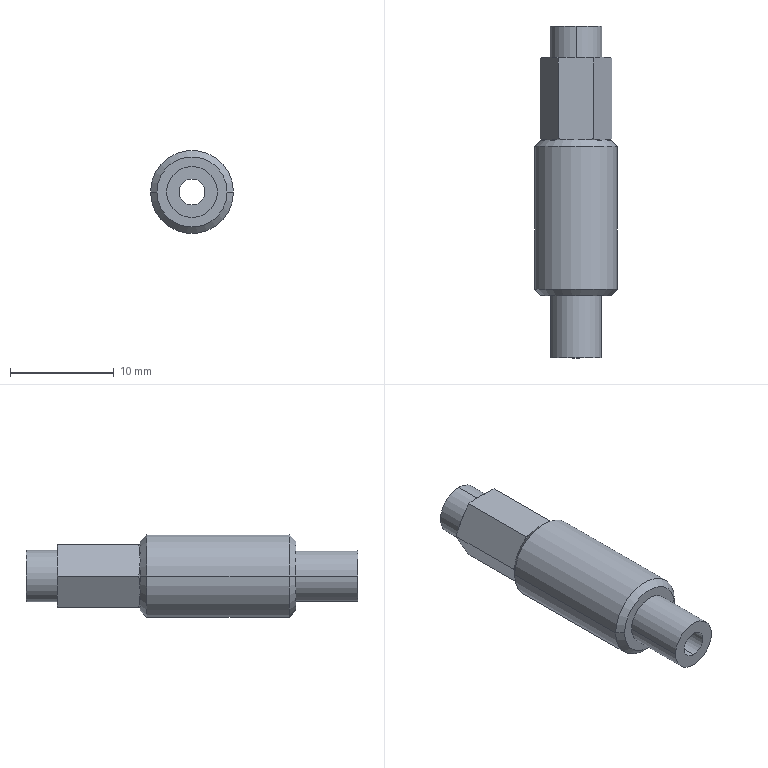Part | SolidWorks | features RefAxis 12, 3DProfileFeature 4, Revolution 2, ICE 1, RevCut 1 | 1 solid | 37 faces | box 8 x 32 x 8 mm | volume 1009 mm3 | cone 18 | plane 11 | cylinder 8 | commonest cylinder face diameters 2.5 x2 4.9 x2 5 x2 8 x2
STEP:
#1=CARTESIAN_POINT('',(0.,12.,-1.25));
#2=VERTEX_POINT('',#1);
#3=CARTESIAN_POINT('',(0.,12.,1.25));
#4=VERTEX_POINT('',#3);
#5=CARTESIAN_POINT('',(0.,12.,0.));
#6=DIRECTION('',(0.,1.,0.));
#7=DIRECTION('',(0.,0.,1.));
#8=AXIS2_PLACEMENT_3D('',#5,#6,#7);
#9=CIRCLE('',#8,1.25);
#10=EDGE_CURVE('',#2,#4,#9,.T.);
#11=ORIENTED_EDGE('',*,*,#10,.F.);
#12=CARTESIAN_POINT('',(0.,44.,-1.25));
#13=VERTEX_POINT('',#12);
#14=CARTESIAN_POINT('',(0.,12.,-1.25));
#15=DIRECTION('',(0.,1.,0.));
#16=VECTOR('',#15,1000.);
#17=LINE('',#14,#16);
#18=EDGE_CURVE('',#2,#13,#17,.T.);
#19=ORIENTED_EDGE('',*,*,#18,.T.);
#20=CARTESIAN_POINT('',(0.,44.,1.25));
#21=VERTEX_POINT('',#20);
#22=CARTESIAN_POINT('',(0.,44.,0.));
#23=DIRECTION('',(0.,1.,0.));
#24=DIRECTION('',(0.,0.,1.));
#25=AXIS2_PLACEMENT_3D('',#22,#23,#24);
#26=CIRCLE('',#25,1.25);
#27=EDGE_CURVE('',#13,#21,#26,.T.);
#28=ORIENTED_EDGE('',*,*,#27,.T.);
#29=CARTESIAN_POINT('',(0.,12.,1.25));
#30=DIRECTION('',(0.,1.,0.));
#31=VECTOR('',#30,1000.);
#32=LINE('',#29,#31);
#33=EDGE_CURVE('',#4,#21,#32,.T.);
#34=ORIENTED_EDGE('',*,*,#33,.F.);
#35=EDGE_LOOP('',(#11,#19,#28,#34));
#36=FACE_OUTER_BOUND('',#35,.T.);
#37=CARTESIAN_POINT('',(0.,12.,0.));
#38=DIRECTION('',(0.,1.,0.));
#39=DIRECTION('',(0.,0.,1.));
#40=AXIS2_PLACEMENT_3D('',#37,#38,#39);
#41=CYLINDRICAL_SURFACE('',#40,1.25);
#42=ADVANCED_FACE('',(#36),#41,.F.);
#43=CARTESIAN_POINT('',(0.,41.,2.5));
#44=VERTEX_POINT('',#43);
#45=CARTESIAN_POINT('',(0.,41.,-2.5));
#46=VERTEX_POINT('',#45);
#47=CARTESIAN_POINT('',(0.,41.,0.));
#48=DIRECTION('',(0.,1.,0.));
#49=DIRECTION('',(1.,0.,0.));
#50=AXIS2_PLACEMENT_3D('',#47,#48,#49);
#51=CIRCLE('',#50,2.5);
#52=EDGE_CURVE('',#44,#46,#51,.T.);
#53=ORIENTED_EDGE('',*,*,#52,.T.);
#54=CARTESIAN_POINT('',(0.,44.,-2.5));
#55=VERTEX_POINT('',#54);
#56=CARTESIAN_POINT('',(0.,41.,-2.5));
#57=DIRECTION('',(0.,1.,0.));
#58=VECTOR('',#57,1000.);
#59=LINE('',#56,#58);
#60=EDGE_CURVE('',#46,#55,#59,.T.);
#61=ORIENTED_EDGE('',*,*,#60,.T.);
#62=CARTESIAN_POINT('',(0.,44.,2.5));
#63=VERTEX_POINT('',#62);
#64=CARTESIAN_POINT('',(0.,44.,0.));
#65=DIRECTION('',(0.,1.,0.));
#66=DIRECTION('',(0.,0.,1.));
#67=AXIS2_PLACEMENT_3D('',#64,#65,#66);
#68=CIRCLE('',#67,2.5);
#69=EDGE_CURVE('',#63,#55,#68,.T.);
#70=ORIENTED_EDGE('',*,*,#69,.F.);
#71=CARTESIAN_POINT('',(0.,41.,2.5));
#72=DIRECTION('',(0.,1.,0.));
#73=VECTOR('',#72,1000.);
#74=LINE('',#71,#73);
#75=EDGE_CURVE('',#44,#63,#74,.T.);
#76=ORIENTED_EDGE('',*,*,#75,.F.);
#77=EDGE_LOOP('',(#53,#61,#70,#76));
#78=FACE_OUTER_BOUND('',#77,.T.);
#79=CARTESIAN_POINT('',(0.,41.,0.));
#80=DIRECTION('',(0.,1.,0.));
#81=DIRECTION('',(0.,0.,1.));
#82=AXIS2_PLACEMENT_3D('',#79,#80,#81);
#83=CYLINDRICAL_SURFACE('',#82,2.5);
#84=ADVANCED_FACE('',(#78),#83,.T.);
#85=CARTESIAN_POINT('',(3.,41.,0.));
#86=VERTEX_POINT('',#85);
#87=CARTESIAN_POINT('',(2.598,41.,-1.5));
#88=VERTEX_POINT('',#87);
#89=CARTESIAN_POINT('',(0.,41.,0.));
#90=DIRECTION('',(0.,1.,0.));
#91=DIRECTION('',(-1.,0.,0.));
#92=AXIS2_PLACEMENT_3D('',#89,#90,#91);
#93=CIRCLE('',#92,3.);
#94=EDGE_CURVE('',#86,#88,#93,.T.);
#95=ORIENTED_EDGE('',*,*,#94,.F.);
#96=CARTESIAN_POINT('',(3.464,40.918,0.));
#97=VERTEX_POINT('',#96);
#98=CARTESIAN_POINT('',(5.,40.647,0.));
#99=DIRECTION('',(0.9848,-0.1736,0.));
#100=VECTOR('',#99,1000.);
#101=LINE('',#98,#100);
#102=EDGE_CURVE('',#86,#97,#101,.T.);
#103=ORIENTED_EDGE('',*,*,#102,.T.);
#104=CARTESIAN_POINT('',(3.464,40.918,0.));
#105=CARTESIAN_POINT('',(3.175,40.969,-0.5));
#106=CARTESIAN_POINT('',(2.887,41.,-1.));
#107=CARTESIAN_POINT('',(2.598,41.,-1.5));
#108=B_SPLINE_CURVE_WITH_KNOTS('',3,(#104,#105,#106,#107),.UNSPECIFIED.,.F.,.F.,(4,4),(0.000000231,0.001732),.UNSPECIFIED.);
#109=EDGE_CURVE('',#97,#88,#108,.T.);
#110=ORIENTED_EDGE('',*,*,#109,.T.);
#111=EDGE_LOOP('',(#95,#103,#110));
#112=FACE_OUTER_BOUND('',#111,.T.);
#113=CARTESIAN_POINT('',(0.,40.647,0.));
#114=DIRECTION('',(0.,-1.,0.));
#115=DIRECTION('',(1.,0.,0.));
#116=AXIS2_PLACEMENT_3D('',#113,#114,#115);
#117=CONICAL_SURFACE('',#116,5.,1.396);
#118=ADVANCED_FACE('',(#112),#117,.T.);
#119=CARTESIAN_POINT('',(-2.45,12.,0.));
#120=VERTEX_POINT('',#119);
#121=CARTESIAN_POINT('',(2.45,12.,0.));
#122=VERTEX_POINT('',#121);
#123=CARTESIAN_POINT('',(0.,12.,0.));
#124=DIRECTION('',(0.,1.,0.));
#125=DIRECTION('',(-1.,0.,0.));
#126=AXIS2_PLACEMENT_3D('',#123,#124,#125);
#127=CIRCLE('',#126,2.45);
#128=EDGE_CURVE('',#120,#122,#127,.T.);
#129=ORIENTED_EDGE('',*,*,#128,.T.);
#130=CARTESIAN_POINT('',(2.45,18.,0.));
#131=VERTEX_POINT('',#130);
#132=CARTESIAN_POINT('',(2.45,12.,0.));
#133=DIRECTION('',(0.,1.,0.));
#134=VECTOR('',#133,1000.);
#135=LINE('',#132,#134);
#136=EDGE_CURVE('',#122,#131,#135,.T.);
#137=ORIENTED_EDGE('',*,*,#136,.T.);
#138=CARTESIAN_POINT('',(-2.45,18.,0.));
#139=VERTEX_POINT('',#138);
#140=CARTESIAN_POINT('',(0.,18.,0.));
#141=DIRECTION('',(0.,1.,0.));
#142=DIRECTION('',(-1.,0.,0.));
#143=AXIS2_PLACEMENT_3D('',#140,#141,#142);
#144=CIRCLE('',#143,2.45);
#145=EDGE_CURVE('',#139,#131,#144,.T.);
#146=ORIENTED_EDGE('',*,*,#145,.F.);
#147=CARTESIAN_POINT('',(-2.45,12.,0.));
#148=DIRECTION('',(0.,1.,0.));
#149=VECTOR('',#148,1000.);
#150=LINE('',#147,#149);
#151=EDGE_CURVE('',#120,#139,#150,.T.);
#152=ORIENTED_EDGE('',*,*,#151,.F.);
#153=EDGE_LOOP('',(#129,#137,#146,#152));
#154=FACE_OUTER_BOUND('',#153,.T.);
#155=CARTESIAN_POINT('',(0.,12.,0.));
#156=DIRECTION('',(0.,1.,0.));
#157=DIRECTION('',(-1.,0.,0.));
#158=AXIS2_PLACEMENT_3D('',#155,#156,#157);
#159=CYLINDRICAL_SURFACE('',#158,2.45);
#160=ADVANCED_FACE('',(#154),#159,.T.);
#161=CARTESIAN_POINT('',(-3.387,18.,0.));
#162=VERTEX_POINT('',#161);
#163=CARTESIAN_POINT('',(3.386,18.,0.));
#164=VERTEX_POINT('',#163);
#165=CARTESIAN_POINT('',(0.,18.,0.));
#166=DIRECTION('',(0.,1.,0.));
#167=DIRECTION('',(-1.,0.,0.));
#168=AXIS2_PLACEMENT_3D('',#165,#166,#167);
#169=CIRCLE('',#168,3.387);
#170=EDGE_CURVE('',#162,#164,#169,.T.);
#171=ORIENTED_EDGE('',*,*,#170,.T.);
#172=CARTESIAN_POINT('',(4.,18.614,0.));
#173=VERTEX_POINT('',#172);
#174=CARTESIAN_POINT('',(3.386,18.,0.));
#175=DIRECTION('',(0.7071,0.7071,0.));
#176=VECTOR('',#175,1000.);
#177=LINE('',#174,#176);
#178=EDGE_CURVE('',#164,#173,#177,.T.);
#179=ORIENTED_EDGE('',*,*,#178,.T.);
#180=CARTESIAN_POINT('',(-4.,18.614,0.));
#181=VERTEX_POINT('',#180);
#182=CARTESIAN_POINT('',(0.,18.614,0.));
#183=DIRECTION('',(0.,1.,0.));
#184=DIRECTION('',(-1.,0.,0.));
#185=AXIS2_PLACEMENT_3D('',#182,#183,#184);
#186=CIRCLE('',#185,4.);
#187=EDGE_CURVE('',#181,#173,#186,.T.);
#188=ORIENTED_EDGE('',*,*,#187,.F.);
#189=CARTESIAN_POINT('',(-3.387,18.,0.));
#190=DIRECTION('',(-0.7071,0.7071,0.));
#191=VECTOR('',#190,1000.);
#192=LINE('',#189,#191);
#193=EDGE_CURVE('',#162,#181,#192,.T.);
#194=ORIENTED_EDGE('',*,*,#193,.F.);
#195=EDGE_LOOP('',(#171,#179,#188,#194));
#196=FACE_OUTER_BOUND('',#195,.T.);
#197=CARTESIAN_POINT('',(0.,18.,0.));
#198=DIRECTION('',(0.,1.,0.));
#199=DIRECTION('',(-1.,0.,0.));
#200=AXIS2_PLACEMENT_3D('',#197,#198,#199);
#201=CONICAL_SURFACE('',#200,3.387,0.7854);
#202=ADVANCED_FACE('',(#196),#201,.T.);
#203=ORIENTED_EDGE('',*,*,#187,.T.);
#204=CARTESIAN_POINT('',(4.,32.386,0.));
#205=VERTEX_POINT('',#204);
#206=CARTESIAN_POINT('',(4.,12.,0.));
#207=DIRECTION('',(0.,1.,0.));
#208=VECTOR('',#207,1000.);
#209=LINE('',#206,#208);
#210=EDGE_CURVE('',#173,#205,#209,.T.);
#211=ORIENTED_EDGE('',*,*,#210,.T.);
#212=CARTESIAN_POINT('',(-4.,32.386,0.));
#213=VERTEX_POINT('',#212);
#214=CARTESIAN_POINT('',(0.,32.386,0.));
#215=DIRECTION('',(0.,1.,0.));
#216=DIRECTION('',(-1.,0.,0.));
#217=AXIS2_PLACEMENT_3D('',#214,#215,#216);
#218=CIRCLE('',#217,4.);
#219=EDGE_CURVE('',#213,#205,#218,.T.);
#220=ORIENTED_EDGE('',*,*,#219,.F.);
#221=CARTESIAN_POINT('',(-4.,12.,0.));
#222=DIRECTION('',(0.,1.,0.));
#223=VECTOR('',#222,1000.);
#224=LINE('',#221,#223);
#225=EDGE_CURVE('',#181,#213,#224,.T.);
#226=ORIENTED_EDGE('',*,*,#225,.F.);
#227=EDGE_LOOP('',(#203,#211,#220,#226));
#228=FACE_OUTER_BOUND('',#227,.T.);
#229=CARTESIAN_POINT('',(0.,12.,0.));
#230=DIRECTION('',(0.,1.,0.));
#231=DIRECTION('',(-1.,0.,0.));
#232=AXIS2_PLACEMENT_3D('',#229,#230,#231);
#233=CYLINDRICAL_SURFACE('',#232,4.);
#234=ADVANCED_FACE('',(#228),#233,.T.);
#235=CARTESIAN_POINT('',(-3.387,33.,0.));
#236=VERTEX_POINT('',#235);
#237=CARTESIAN_POINT('',(3.387,33.,0.));
#238=VERTEX_POINT('',#237);
#239=CARTESIAN_POINT('',(0.,33.,0.));
#240=DIRECTION('',(0.,1.,0.));
#241=DIRECTION('',(-1.,0.,0.));
#242=AXIS2_PLACEMENT_3D('',#239,#240,#241);
#243=CIRCLE('',#242,3.387);
#244=EDGE_CURVE('',#236,#238,#243,.T.);
#245=ORIENTED_EDGE('',*,*,#244,.F.);
#246=CARTESIAN_POINT('',(-4.,32.386,0.));
#247=DIRECTION('',(-0.7071,-0.7071,0.));
#248=VECTOR('',#247,1000.);
#249=LINE('',#246,#248);
#250=EDGE_CURVE('',#236,#213,#249,.T.);
#251=ORIENTED_EDGE('',*,*,#250,.T.);
#252=ORIENTED_EDGE('',*,*,#219,.T.);
#253=CARTESIAN_POINT('',(4.,32.386,0.));
#254=DIRECTION('',(0.7071,-0.7071,0.));
#255=VECTOR('',#254,1000.);
#256=LINE('',#253,#255);
#257=EDGE_CURVE('',#238,#205,#256,.T.);
#258=ORIENTED_EDGE('',*,*,#257,.F.);
#259=EDGE_LOOP('',(#245,#251,#252,#258));
#260=FACE_OUTER_BOUND('',#259,.T.);
#261=CARTESIAN_POINT('',(0.,32.386,0.));
#262=DIRECTION('',(0.,-1.,0.));
#263=DIRECTION('',(1.,0.,0.));
#264=AXIS2_PLACEMENT_3D('',#261,#262,#263);
#265=CONICAL_SURFACE('',#264,4.,0.7854);
#266=ADVANCED_FACE('',(#260),#265,.T.);
#267=CARTESIAN_POINT('',(-2.598,33.,-1.5));
#268=VERTEX_POINT('',#267);
#269=CARTESIAN_POINT('',(-3.,33.,0.));
#270=VERTEX_POINT('',#269);
#271=CARTESIAN_POINT('',(0.,33.,0.));
#272=DIRECTION('',(0.,1.,0.));
#273=DIRECTION('',(-1.,0.,0.));
#274=AXIS2_PLACEMENT_3D('',#271,#272,#273);
#275=CIRCLE('',#274,3.);
#276=EDGE_CURVE('',#268,#270,#275,.T.);
#277=ORIENTED_EDGE('',*,*,#276,.T.);
#278=CARTESIAN_POINT('',(-3.464,33.124,0.));
#279=VERTEX_POINT('',#278);
#280=CARTESIAN_POINT('',(-3.,33.,0.));
#281=DIRECTION('',(-0.9659,0.2588,0.));
#282=VECTOR('',#281,1000.);
#283=LINE('',#280,#282);
#284=EDGE_CURVE('',#270,#279,#283,.T.);
#285=ORIENTED_EDGE('',*,*,#284,.T.);
#286=CARTESIAN_POINT('',(-3.464,33.124,0.));
#287=CARTESIAN_POINT('',(-3.175,33.047,-0.5));
#288=CARTESIAN_POINT('',(-2.887,33.,-1.));
#289=CARTESIAN_POINT('',(-2.598,33.,-1.5));
#290=B_SPLINE_CURVE_WITH_KNOTS('',3,(#286,#287,#288,#289),.UNSPECIFIED.,.F.,.F.,(4,4),(0.000000231,0.001732),.UNSPECIFIED.);
#291=EDGE_CURVE('',#279,#268,#290,.T.);
#292=ORIENTED_EDGE('',*,*,#291,.T.);
#293=EDGE_LOOP('',(#277,#285,#292));
#294=FACE_OUTER_BOUND('',#293,.T.);
#295=CARTESIAN_POINT('',(0.,33.,0.));
#296=DIRECTION('',(0.,1.,0.));
#297=DIRECTION('',(-1.,0.,0.));
#298=AXIS2_PLACEMENT_3D('',#295,#296,#297);
#299=CONICAL_SURFACE('',#298,3.,1.309);
#300=ADVANCED_FACE('',(#294),#299,.T.);
#301=ORIENTED_EDGE('',*,*,#128,.F.);
#302=CARTESIAN_POINT('',(0.,12.,0.));
#303=DIRECTION('',(0.,1.,0.));
#304=DIRECTION('',(-1.,0.,0.));
#305=AXIS2_PLACEMENT_3D('',#302,#303,#304);
#306=CIRCLE('',#305,2.45);
#307=EDGE_CURVE('',#122,#120,#306,.T.);
#308=ORIENTED_EDGE('',*,*,#307,.F.);
#309=EDGE_LOOP('',(#301,#308));
#310=FACE_OUTER_BOUND('',#309,.T.);
#311=CARTESIAN_POINT('',(0.,12.,0.));
#312=DIRECTION('',(0.,1.,0.));
#313=DIRECTION('',(0.,0.,1.));
#314=AXIS2_PLACEMENT_3D('',#311,#312,#313);
#315=CIRCLE('',#314,1.25);
#316=EDGE_CURVE('',#4,#2,#315,.T.);
#317=ORIENTED_EDGE('',*,*,#316,.T.);
#318=ORIENTED_EDGE('',*,*,#10,.T.);
#319=EDGE_LOOP('',(#317,#318));
#320=FACE_BOUND('',#319,.T.);
#321=CARTESIAN_POINT('',(2.45,12.,0.));
#322=DIRECTION('',(0.,1.,0.));
#323=DIRECTION('',(-1.,0.,0.));
#324=AXIS2_PLACEMENT_3D('',#321,#322,#323);
#325=PLANE('',#324);
#326=ADVANCED_FACE('',(#310,#320),#325,.F.);
#327=ORIENTED_EDGE('',*,*,#69,.T.);
#328=CARTESIAN_POINT('',(0.,44.,0.));
#329=DIRECTION('',(0.,1.,0.));
#330=DIRECTION('',(0.,0.,1.));
#331=AXIS2_PLACEMENT_3D('',#328,#329,#330);
#332=CIRCLE('',#331,2.5);
#333=EDGE_CURVE('',#55,#63,#332,.T.);
#334=ORIENTED_EDGE('',*,*,#333,.T.);
#335=EDGE_LOOP('',(#327,#334));
#336=FACE_OUTER_BOUND('',#335,.T.);
#337=CARTESIAN_POINT('',(0.,44.,0.));
#338=DIRECTION('',(0.,1.,0.));
#339=DIRECTION('',(0.,0.,1.));
#340=AXIS2_PLACEMENT_3D('',#337,#338,#339);
#341=CIRCLE('',#340,1.25);
#342=EDGE_CURVE('',#21,#13,#341,.T.);
#343=ORIENTED_EDGE('',*,*,#342,.F.);
#344=ORIENTED_EDGE('',*,*,#27,.F.);
#345=EDGE_LOOP('',(#343,#344));
#346=FACE_BOUND('',#345,.T.);
#347=CARTESIAN_POINT('',(0.,44.,0.));
#348=DIRECTION('',(0.,-1.,0.));
#349=DIRECTION('',(0.,0.,-1.));
#350=AXIS2_PLACEMENT_3D('',#347,#348,#349);
#351=PLANE('',#350);
#352=ADVANCED_FACE('',(#336,#346),#351,.F.);
#353=CARTESIAN_POINT('',(-2.598,41.,1.5));
#354=VERTEX_POINT('',#353);
#355=CARTESIAN_POINT('',(0.,41.,3.));
#356=VERTEX_POINT('',#355);
#357=CARTESIAN_POINT('',(0.,41.,0.));
#358=DIRECTION('',(0.,1.,0.));
#359=DIRECTION('',(-1.,0.,0.));
#360=AXIS2_PLACEMENT_3D('',#357,#358,#359);
#361=CIRCLE('',#360,3.);
#362=EDGE_CURVE('',#354,#356,#361,.T.);
#363=ORIENTED_EDGE('',*,*,#362,.T.);
#364=CARTESIAN_POINT('',(2.598,41.,1.5));
#365=VERTEX_POINT('',#364);
#366=CARTESIAN_POINT('',(0.,41.,0.));
#367=DIRECTION('',(0.,1.,0.));
#368=DIRECTION('',(-1.,0.,0.));
#369=AXIS2_PLACEMENT_3D('',#366,#367,#368);
#370=CIRCLE('',#369,3.);
#371=EDGE_CURVE('',#356,#365,#370,.T.);
#372=ORIENTED_EDGE('',*,*,#371,.T.);
#373=CARTESIAN_POINT('',(0.,41.,0.));
#374=DIRECTION('',(0.,1.,0.));
#375=DIRECTION('',(-1.,0.,0.));
#376=AXIS2_PLACEMENT_3D('',#373,#374,#375);
#377=CIRCLE('',#376,3.);
#378=EDGE_CURVE('',#365,#86,#377,.T.);
#379=ORIENTED_EDGE('',*,*,#378,.T.);
#380=ORIENTED_EDGE('',*,*,#94,.T.);
#381=CARTESIAN_POINT('',(0.,41.,-3.));
#382=VERTEX_POINT('',#381);
#383=CARTESIAN_POINT('',(0.,41.,0.));
#384=DIRECTION('',(0.,1.,0.));
#385=DIRECTION('',(-1.,0.,0.));
#386=AXIS2_PLACEMENT_3D('',#383,#384,#385);
#387=CIRCLE('',#386,3.);
#388=EDGE_CURVE('',#88,#382,#387,.T.);
#389=ORIENTED_EDGE('',*,*,#388,.T.);
#390=CARTESIAN_POINT('',(-2.598,41.,-1.5));
#391=VERTEX_POINT('',#390);
#392=CARTESIAN_POINT('',(0.,41.,0.));
#393=DIRECTION('',(0.,1.,0.));
#394=DIRECTION('',(-1.,0.,0.));
#395=AXIS2_PLACEMENT_3D('',#392,#393,#394);
#396=CIRCLE('',#395,3.);
#397=EDGE_CURVE('',#382,#391,#396,.T.);
#398=ORIENTED_EDGE('',*,*,#397,.T.);
#399=CARTESIAN_POINT('',(0.,41.,0.));
#400=DIRECTION('',(0.,1.,0.));
#401=DIRECTION('',(-1.,0.,0.));
#402=AXIS2_PLACEMENT_3D('',#399,#400,#401);
#403=CIRCLE('',#402,3.);
#404=EDGE_CURVE('',#391,#354,#403,.T.);
#405=ORIENTED_EDGE('',*,*,#404,.T.);
#406=EDGE_LOOP('',(#363,#372,#379,#380,#389,#398,#405));
#407=FACE_OUTER_BOUND('',#406,.T.);
#408=ORIENTED_EDGE('',*,*,#52,.F.);
#409=CARTESIAN_POINT('',(0.,41.,0.));
#410=DIRECTION('',(0.,1.,0.));
#411=DIRECTION('',(1.,0.,0.));
#412=AXIS2_PLACEMENT_3D('',#409,#410,#411);
#413=CIRCLE('',#412,2.5);
#414=EDGE_CURVE('',#46,#44,#413,.T.);
#415=ORIENTED_EDGE('',*,*,#414,.F.);
#416=EDGE_LOOP('',(#408,#415));
#417=FACE_BOUND('',#416,.T.);
#418=CARTESIAN_POINT('',(0.,41.,0.));
#419=DIRECTION('',(0.,-1.,0.));
#420=DIRECTION('',(1.,0.,0.));
#421=AXIS2_PLACEMENT_3D('',#418,#419,#420);
#422=PLANE('',#421);
#423=ADVANCED_FACE('',(#407,#417),#422,.F.);
#424=CARTESIAN_POINT('',(2.598,33.,1.5));
#425=VERTEX_POINT('',#424);
#426=CARTESIAN_POINT('',(1.732,33.124,3.));
#427=VERTEX_POINT('',#426);
#428=CARTESIAN_POINT('',(2.598,33.,1.5));
#429=CARTESIAN_POINT('',(2.309,33.,2.));
#430=CARTESIAN_POINT('',(2.021,33.047,2.5));
#431=CARTESIAN_POINT('',(1.732,33.124,3.));
#432=B_SPLINE_CURVE_WITH_KNOTS('',3,(#428,#429,#430,#431),.UNSPECIFIED.,.F.,.F.,(4,4),(0.001732,0.003464),.UNSPECIFIED.);
#433=EDGE_CURVE('',#425,#427,#432,.T.);
#434=ORIENTED_EDGE('',*,*,#433,.T.);
#435=CARTESIAN_POINT('',(0.,33.,3.));
#436=VERTEX_POINT('',#435);
#437=CARTESIAN_POINT('',(1.732,33.124,3.));
#438=CARTESIAN_POINT('',(1.156,33.047,3.));
#439=CARTESIAN_POINT('',(0.5785,33.,3.));
#440=CARTESIAN_POINT('',(0.,33.,3.));
#441=B_SPLINE_CURVE_WITH_KNOTS('',3,(#437,#438,#439,#440),.UNSPECIFIED.,.F.,.F.,(4,4),(0.00677,0.008513),.UNSPECIFIED.);
#442=EDGE_CURVE('',#427,#436,#441,.T.);
#443=ORIENTED_EDGE('',*,*,#442,.T.);
#444=CARTESIAN_POINT('',(0.,33.,0.));
#445=DIRECTION('',(0.,1.,0.));
#446=DIRECTION('',(-1.,0.,0.));
#447=AXIS2_PLACEMENT_3D('',#444,#445,#446);
#448=CIRCLE('',#447,3.);
#449=EDGE_CURVE('',#436,#425,#448,.T.);
#450=ORIENTED_EDGE('',*,*,#449,.T.);
#451=EDGE_LOOP('',(#434,#443,#450));
#452=FACE_OUTER_BOUND('',#451,.T.);
#453=CARTESIAN_POINT('',(0.,33.,0.));
#454=DIRECTION('',(0.,1.,0.));
#455=DIRECTION('',(-1.,0.,0.));
#456=AXIS2_PLACEMENT_3D('',#453,#454,#455);
#457=CONICAL_SURFACE('',#456,3.,1.309);
#458=ADVANCED_FACE('',(#452),#457,.T.);
#459=CARTESIAN_POINT('',(-2.598,33.,1.5));
#460=VERTEX_POINT('',#459);
#461=CARTESIAN_POINT('',(0.,33.,0.));
#462=DIRECTION('',(0.,1.,0.));
#463=DIRECTION('',(-1.,0.,0.));
#464=AXIS2_PLACEMENT_3D('',#461,#462,#463);
#465=CIRCLE('',#464,3.);
#466=EDGE_CURVE('',#460,#436,#465,.T.);
#467=ORIENTED_EDGE('',*,*,#466,.T.);
#468=CARTESIAN_POINT('',(-1.732,33.124,3.));
#469=VERTEX_POINT('',#468);
#470=CARTESIAN_POINT('',(0.,33.,3.));
#471=CARTESIAN_POINT('',(-0.5766,33.,3.));
#472=CARTESIAN_POINT('',(-1.156,33.047,3.));
#473=CARTESIAN_POINT('',(-1.732,33.124,3.));
#474=B_SPLINE_CURVE_WITH_KNOTS('',3,(#470,#471,#472,#473),.UNSPECIFIED.,.F.,.F.,(4,4),(0.008513,0.01025),.UNSPECIFIED.);
#475=EDGE_CURVE('',#436,#469,#474,.T.);
#476=ORIENTED_EDGE('',*,*,#475,.T.);
#477=CARTESIAN_POINT('',(-1.732,33.124,3.));
#478=CARTESIAN_POINT('',(-2.021,33.047,2.5));
#479=CARTESIAN_POINT('',(-2.309,33.,2.));
#480=CARTESIAN_POINT('',(-2.598,33.,1.5));
#481=B_SPLINE_CURVE_WITH_KNOTS('',3,(#477,#478,#479,#480),.UNSPECIFIED.,.F.,.F.,(4,4),(0.000000231,0.001732),.UNSPECIFIED.);
#482=EDGE_CURVE('',#469,#460,#481,.T.);
#483=ORIENTED_EDGE('',*,*,#482,.T.);
#484=EDGE_LOOP('',(#467,#476,#483));
#485=FACE_OUTER_BOUND('',#484,.T.);
#486=CARTESIAN_POINT('',(0.,33.,0.));
#487=DIRECTION('',(0.,1.,0.));
#488=DIRECTION('',(-1.,0.,0.));
#489=AXIS2_PLACEMENT_3D('',#486,#487,#488);
#490=CONICAL_SURFACE('',#489,3.,1.309);
#491=ADVANCED_FACE('',(#485),#490,.T.);
#492=ORIENTED_EDGE('',*,*,#284,.F.);
#493=CARTESIAN_POINT('',(0.,33.,0.));
#494=DIRECTION('',(0.,1.,0.));
#495=DIRECTION('',(-1.,0.,0.));
#496=AXIS2_PLACEMENT_3D('',#493,#494,#495);
#497=CIRCLE('',#496,3.);
#498=EDGE_CURVE('',#270,#460,#497,.T.);
#499=ORIENTED_EDGE('',*,*,#498,.T.);
#500=CARTESIAN_POINT('',(-2.598,33.,1.5));
#501=CARTESIAN_POINT('',(-2.887,33.,1.));
#502=CARTESIAN_POINT('',(-3.175,33.047,0.5));
#503=CARTESIAN_POINT('',(-3.464,33.124,0.));
#504=B_SPLINE_CURVE_WITH_KNOTS('',3,(#500,#501,#502,#503),.UNSPECIFIED.,.F.,.F.,(4,4),(0.001732,0.003464),.UNSPECIFIED.);
#505=EDGE_CURVE('',#460,#279,#504,.T.);
#506=ORIENTED_EDGE('',*,*,#505,.T.);
#507=EDGE_LOOP('',(#492,#499,#506));
#508=FACE_OUTER_BOUND('',#507,.T.);
#509=CARTESIAN_POINT('',(0.,33.,0.));
#510=DIRECTION('',(0.,1.,0.));
#511=DIRECTION('',(-1.,0.,0.));
#512=AXIS2_PLACEMENT_3D('',#509,#510,#511);
#513=CONICAL_SURFACE('',#512,3.,1.309);
#514=ADVANCED_FACE('',(#508),#513,.T.);
#515=CARTESIAN_POINT('',(2.598,33.,-1.5));
#516=VERTEX_POINT('',#515);
#517=CARTESIAN_POINT('',(3.464,33.124,0.));
#518=VERTEX_POINT('',#517);
#519=CARTESIAN_POINT('',(2.598,33.,-1.5));
#520=CARTESIAN_POINT('',(2.887,33.,-1.));
#521=CARTESIAN_POINT('',(3.175,33.047,-0.5));
#522=CARTESIAN_POINT('',(3.464,33.124,0.));
#523=B_SPLINE_CURVE_WITH_KNOTS('',3,(#519,#520,#521,#522),.UNSPECIFIED.,.F.,.F.,(4,4),(0.001732,0.003464),.UNSPECIFIED.);
#524=EDGE_CURVE('',#516,#518,#523,.T.);
#525=ORIENTED_EDGE('',*,*,#524,.T.);
#526=CARTESIAN_POINT('',(3.464,33.124,0.));
#527=CARTESIAN_POINT('',(3.175,33.047,0.5));
#528=CARTESIAN_POINT('',(2.887,33.,1.));
#529=CARTESIAN_POINT('',(2.598,33.,1.5));
#530=B_SPLINE_CURVE_WITH_KNOTS('',3,(#526,#527,#528,#529),.UNSPECIFIED.,.F.,.F.,(4,4),(0.000000231,0.001732),.UNSPECIFIED.);
#531=EDGE_CURVE('',#518,#425,#530,.T.);
#532=ORIENTED_EDGE('',*,*,#531,.T.);
#533=CARTESIAN_POINT('',(0.,33.,0.));
#534=DIRECTION('',(0.,1.,0.));
#535=DIRECTION('',(-1.,0.,0.));
#536=AXIS2_PLACEMENT_3D('',#533,#534,#535);
#537=CIRCLE('',#536,3.);
#538=EDGE_CURVE('',#425,#516,#537,.T.);
#539=ORIENTED_EDGE('',*,*,#538,.T.);
#540=EDGE_LOOP('',(#525,#532,#539));
#541=FACE_OUTER_BOUND('',#540,.T.);
#542=CARTESIAN_POINT('',(0.,33.,0.));
#543=DIRECTION('',(0.,1.,0.));
#544=DIRECTION('',(-1.,0.,0.));
#545=AXIS2_PLACEMENT_3D('',#542,#543,#544);
#546=CONICAL_SURFACE('',#545,3.,1.309);
#547=ADVANCED_FACE('',(#541),#546,.T.);
#548=CARTESIAN_POINT('',(0.,33.,-3.));
#549=VERTEX_POINT('',#548);
#550=CARTESIAN_POINT('',(0.,33.,0.));
#551=DIRECTION('',(0.,1.,0.));
#552=DIRECTION('',(-1.,0.,0.));
#553=AXIS2_PLACEMENT_3D('',#550,#551,#552);
#554=CIRCLE('',#553,3.);
#555=EDGE_CURVE('',#549,#268,#554,.T.);
#556=ORIENTED_EDGE('',*,*,#555,.T.);
#557=CARTESIAN_POINT('',(-1.732,33.124,-3.));
#558=VERTEX_POINT('',#557);
#559=CARTESIAN_POINT('',(-2.598,33.,-1.5));
#560=CARTESIAN_POINT('',(-2.309,33.,-2.));
#561=CARTESIAN_POINT('',(-2.021,33.047,-2.5));
#562=CARTESIAN_POINT('',(-1.732,33.124,-3.));
#563=B_SPLINE_CURVE_WITH_KNOTS('',3,(#559,#560,#561,#562),.UNSPECIFIED.,.F.,.F.,(4,4),(0.001732,0.003464),.UNSPECIFIED.);
#564=EDGE_CURVE('',#268,#558,#563,.T.);
#565=ORIENTED_EDGE('',*,*,#564,.T.);
#566=CARTESIAN_POINT('',(-1.732,33.124,-3.));
#567=CARTESIAN_POINT('',(-1.156,33.047,-3.));
#568=CARTESIAN_POINT('',(-0.5766,33.,-3.));
#569=CARTESIAN_POINT('',(0.,33.,-3.));
#570=B_SPLINE_CURVE_WITH_KNOTS('',3,(#566,#567,#568,#569),.UNSPECIFIED.,.F.,.F.,(4,4),(0.002928,0.004669),.UNSPECIFIED.);
#571=EDGE_CURVE('',#558,#549,#570,.T.);
#572=ORIENTED_EDGE('',*,*,#571,.T.);
#573=EDGE_LOOP('',(#556,#565,#572));
#574=FACE_OUTER_BOUND('',#573,.T.);
#575=CARTESIAN_POINT('',(0.,33.,0.));
#576=DIRECTION('',(0.,1.,0.));
#577=DIRECTION('',(-1.,0.,0.));
#578=AXIS2_PLACEMENT_3D('',#575,#576,#577);
#579=CONICAL_SURFACE('',#578,3.,1.309);
#580=ADVANCED_FACE('',(#574),#579,.T.);
#581=CARTESIAN_POINT('',(1.732,33.124,-3.));
#582=VERTEX_POINT('',#581);
#583=CARTESIAN_POINT('',(0.,33.,-3.));
#584=CARTESIAN_POINT('',(0.5785,33.,-3.));
#585=CARTESIAN_POINT('',(1.156,33.047,-3.));
#586=CARTESIAN_POINT('',(1.732,33.124,-3.));
#587=B_SPLINE_CURVE_WITH_KNOTS('',3,(#583,#584,#585,#586),.UNSPECIFIED.,.F.,.F.,(4,4),(0.004669,0.006415),.UNSPECIFIED.);
#588=EDGE_CURVE('',#549,#582,#587,.T.);
#589=ORIENTED_EDGE('',*,*,#588,.T.);
#590=CARTESIAN_POINT('',(1.732,33.124,-3.));
#591=CARTESIAN_POINT('',(2.021,33.047,-2.5));
#592=CARTESIAN_POINT('',(2.309,33.,-2.));
#593=CARTESIAN_POINT('',(2.598,33.,-1.5));
#594=B_SPLINE_CURVE_WITH_KNOTS('',3,(#590,#591,#592,#593),.UNSPECIFIED.,.F.,.F.,(4,4),(0.000000231,0.001732),.UNSPECIFIED.);
#595=EDGE_CURVE('',#582,#516,#594,.T.);
#596=ORIENTED_EDGE('',*,*,#595,.T.);
#597=CARTESIAN_POINT('',(0.,33.,0.));
#598=DIRECTION('',(0.,1.,0.));
#599=DIRECTION('',(-1.,0.,0.));
#600=AXIS2_PLACEMENT_3D('',#597,#598,#599);
#601=CIRCLE('',#600,3.);
#602=EDGE_CURVE('',#516,#549,#601,.T.);
#603=ORIENTED_EDGE('',*,*,#602,.T.);
#604=EDGE_LOOP('',(#589,#596,#603));
#605=FACE_OUTER_BOUND('',#604,.T.);
#606=CARTESIAN_POINT('',(0.,33.,0.));
#607=DIRECTION('',(0.,1.,0.));
#608=DIRECTION('',(-1.,0.,0.));
#609=AXIS2_PLACEMENT_3D('',#606,#607,#608);
#610=CONICAL_SURFACE('',#609,3.,1.309);
#611=ADVANCED_FACE('',(#605),#610,.T.);
#612=ORIENTED_EDGE('',*,*,#276,.F.);
#613=ORIENTED_EDGE('',*,*,#555,.F.);
#614=ORIENTED_EDGE('',*,*,#602,.F.);
#615=ORIENTED_EDGE('',*,*,#538,.F.);
#616=ORIENTED_EDGE('',*,*,#449,.F.);
#617=ORIENTED_EDGE('',*,*,#466,.F.);
#618=ORIENTED_EDGE('',*,*,#498,.F.);
#619=EDGE_LOOP('',(#612,#613,#614,#615,#616,#617,#618));
#620=FACE_BOUND('',#619,.T.);
#621=CARTESIAN_POINT('',(0.,33.,0.));
#622=DIRECTION('',(0.,1.,0.));
#623=DIRECTION('',(-1.,0.,0.));
#624=AXIS2_PLACEMENT_3D('',#621,#622,#623);
#625=CIRCLE('',#624,3.387);
#626=EDGE_CURVE('',#238,#236,#625,.T.);
#627=ORIENTED_EDGE('',*,*,#626,.T.);
#628=ORIENTED_EDGE('',*,*,#244,.T.);
#629=EDGE_LOOP('',(#627,#628));
#630=FACE_OUTER_BOUND('',#629,.T.);
#631=CARTESIAN_POINT('',(3.,33.,0.));
#632=DIRECTION('',(0.,-1.,0.));
#633=DIRECTION('',(1.,0.,0.));
#634=AXIS2_PLACEMENT_3D('',#631,#632,#633);
#635=PLANE('',#634);
#636=ADVANCED_FACE('',(#620,#630),#635,.F.);
#637=ORIENTED_EDGE('',*,*,#250,.F.);
#638=ORIENTED_EDGE('',*,*,#626,.F.);
#639=ORIENTED_EDGE('',*,*,#257,.T.);
#640=CARTESIAN_POINT('',(0.,32.386,0.));
#641=DIRECTION('',(0.,1.,0.));
#642=DIRECTION('',(-1.,0.,0.));
#643=AXIS2_PLACEMENT_3D('',#640,#641,#642);
#644=CIRCLE('',#643,4.);
#645=EDGE_CURVE('',#205,#213,#644,.T.);
#646=ORIENTED_EDGE('',*,*,#645,.T.);
#647=EDGE_LOOP('',(#637,#638,#639,#646));
#648=FACE_OUTER_BOUND('',#647,.T.);
#649=CARTESIAN_POINT('',(0.,32.386,0.));
#650=DIRECTION('',(0.,-1.,0.));
#651=DIRECTION('',(1.,0.,0.));
#652=AXIS2_PLACEMENT_3D('',#649,#650,#651);
#653=CONICAL_SURFACE('',#652,4.,0.7854);
#654=ADVANCED_FACE('',(#648),#653,.T.);
#655=ORIENTED_EDGE('',*,*,#210,.F.);
#656=CARTESIAN_POINT('',(0.,18.614,0.));
#657=DIRECTION('',(0.,1.,0.));
#658=DIRECTION('',(-1.,0.,0.));
#659=AXIS2_PLACEMENT_3D('',#656,#657,#658);
#660=CIRCLE('',#659,4.);
#661=EDGE_CURVE('',#173,#181,#660,.T.);
#662=ORIENTED_EDGE('',*,*,#661,.T.);
#663=ORIENTED_EDGE('',*,*,#225,.T.);
#664=ORIENTED_EDGE('',*,*,#645,.F.);
#665=EDGE_LOOP('',(#655,#662,#663,#664));
#666=FACE_OUTER_BOUND('',#665,.T.);
#667=CARTESIAN_POINT('',(0.,12.,0.));
#668=DIRECTION('',(0.,1.,0.));
#669=DIRECTION('',(-1.,0.,0.));
#670=AXIS2_PLACEMENT_3D('',#667,#668,#669);
#671=CYLINDRICAL_SURFACE('',#670,4.);
#672=ADVANCED_FACE('',(#666),#671,.T.);
#673=ORIENTED_EDGE('',*,*,#178,.F.);
#674=CARTESIAN_POINT('',(0.,18.,0.));
#675=DIRECTION('',(0.,1.,0.));
#676=DIRECTION('',(-1.,0.,0.));
#677=AXIS2_PLACEMENT_3D('',#674,#675,#676);
#678=CIRCLE('',#677,3.387);
#679=EDGE_CURVE('',#164,#162,#678,.T.);
#680=ORIENTED_EDGE('',*,*,#679,.T.);
#681=ORIENTED_EDGE('',*,*,#193,.T.);
#682=ORIENTED_EDGE('',*,*,#661,.F.);
#683=EDGE_LOOP('',(#673,#680,#681,#682));
#684=FACE_OUTER_BOUND('',#683,.T.);
#685=CARTESIAN_POINT('',(0.,18.,0.));
#686=DIRECTION('',(0.,1.,0.));
#687=DIRECTION('',(-1.,0.,0.));
#688=AXIS2_PLACEMENT_3D('',#685,#686,#687);
#689=CONICAL_SURFACE('',#688,3.387,0.7854);
#690=ADVANCED_FACE('',(#684),#689,.T.);
#691=ORIENTED_EDGE('',*,*,#170,.F.);
#692=ORIENTED_EDGE('',*,*,#679,.F.);
#693=EDGE_LOOP('',(#691,#692));
#694=FACE_OUTER_BOUND('',#693,.T.);
#695=ORIENTED_EDGE('',*,*,#145,.T.);
#696=CARTESIAN_POINT('',(0.,18.,0.));
#697=DIRECTION('',(0.,1.,0.));
#698=DIRECTION('',(-1.,0.,0.));
#699=AXIS2_PLACEMENT_3D('',#696,#697,#698);
#700=CIRCLE('',#699,2.45);
#701=EDGE_CURVE('',#131,#139,#700,.T.);
#702=ORIENTED_EDGE('',*,*,#701,.T.);
#703=EDGE_LOOP('',(#695,#702));
#704=FACE_BOUND('',#703,.T.);
#705=CARTESIAN_POINT('',(3.386,18.,0.));
#706=DIRECTION('',(0.,1.,0.));
#707=DIRECTION('',(-1.,0.,0.));
#708=AXIS2_PLACEMENT_3D('',#705,#706,#707);
#709=PLANE('',#708);
#710=ADVANCED_FACE('',(#694,#704),#709,.F.);
#711=ORIENTED_EDGE('',*,*,#136,.F.);
#712=ORIENTED_EDGE('',*,*,#307,.T.);
#713=ORIENTED_EDGE('',*,*,#151,.T.);
#714=ORIENTED_EDGE('',*,*,#701,.F.);
#715=EDGE_LOOP('',(#711,#712,#713,#714));
#716=FACE_OUTER_BOUND('',#715,.T.);
#717=CARTESIAN_POINT('',(0.,12.,0.));
#718=DIRECTION('',(0.,1.,0.));
#719=DIRECTION('',(-1.,0.,0.));
#720=AXIS2_PLACEMENT_3D('',#717,#718,#719);
#721=CYLINDRICAL_SURFACE('',#720,2.45);
#722=ADVANCED_FACE('',(#716),#721,.T.);
#723=CARTESIAN_POINT('',(-1.732,40.918,-3.));
#724=VERTEX_POINT('',#723);
#725=CARTESIAN_POINT('',(-1.732,41.,-3.));
#726=DIRECTION('',(0.,-1.,0.));
#727=VECTOR('',#726,1000.);
#728=LINE('',#725,#727);
#729=EDGE_CURVE('',#724,#558,#728,.T.);
#730=ORIENTED_EDGE('',*,*,#729,.T.);
#731=ORIENTED_EDGE('',*,*,#564,.F.);
#732=ORIENTED_EDGE('',*,*,#291,.F.);
#733=CARTESIAN_POINT('',(-3.464,40.918,0.));
#734=VERTEX_POINT('',#733);
#735=CARTESIAN_POINT('',(-3.464,41.,0.));
#736=DIRECTION('',(0.,-1.,0.));
#737=VECTOR('',#736,1000.);
#738=LINE('',#735,#737);
#739=EDGE_CURVE('',#734,#279,#738,.T.);
#740=ORIENTED_EDGE('',*,*,#739,.F.);
#741=CARTESIAN_POINT('',(-2.598,41.,-1.5));
#742=CARTESIAN_POINT('',(-2.887,41.,-1.));
#743=CARTESIAN_POINT('',(-3.175,40.969,-0.5));
#744=CARTESIAN_POINT('',(-3.464,40.918,0.));
#745=B_SPLINE_CURVE_WITH_KNOTS('',3,(#741,#742,#743,#744),.UNSPECIFIED.,.F.,.F.,(4,4),(0.001732,0.003464),.UNSPECIFIED.);
#746=EDGE_CURVE('',#391,#734,#745,.T.);
#747=ORIENTED_EDGE('',*,*,#746,.F.);
#748=CARTESIAN_POINT('',(-1.732,40.918,-3.));
#749=CARTESIAN_POINT('',(-2.021,40.969,-2.5));
#750=CARTESIAN_POINT('',(-2.309,41.,-2.));
#751=CARTESIAN_POINT('',(-2.598,41.,-1.5));
#752=B_SPLINE_CURVE_WITH_KNOTS('',3,(#748,#749,#750,#751),.UNSPECIFIED.,.F.,.F.,(4,4),(0.000000231,0.001732),.UNSPECIFIED.);
#753=EDGE_CURVE('',#724,#391,#752,.T.);
#754=ORIENTED_EDGE('',*,*,#753,.F.);
#755=EDGE_LOOP('',(#730,#731,#732,#740,#747,#754));
#756=FACE_OUTER_BOUND('',#755,.T.);
#757=CARTESIAN_POINT('',(-1.732,41.,-3.));
#758=DIRECTION('',(0.866,0.,0.5));
#759=DIRECTION('',(0.5,0.,-0.866));
#760=AXIS2_PLACEMENT_3D('',#757,#758,#759);
#761=PLANE('',#760);
#762=ADVANCED_FACE('',(#756),#761,.F.);
#763=ORIENTED_EDGE('',*,*,#739,.T.);
#764=ORIENTED_EDGE('',*,*,#505,.F.);
#765=ORIENTED_EDGE('',*,*,#482,.F.);
#766=CARTESIAN_POINT('',(-1.732,40.918,3.));
#767=VERTEX_POINT('',#766);
#768=CARTESIAN_POINT('',(-1.732,41.,3.));
#769=DIRECTION('',(0.,-1.,0.));
#770=VECTOR('',#769,1000.);
#771=LINE('',#768,#770);
#772=EDGE_CURVE('',#767,#469,#771,.T.);
#773=ORIENTED_EDGE('',*,*,#772,.F.);
#774=CARTESIAN_POINT('',(-2.598,41.,1.5));
#775=CARTESIAN_POINT('',(-2.309,41.,2.));
#776=CARTESIAN_POINT('',(-2.021,40.969,2.5));
#777=CARTESIAN_POINT('',(-1.732,40.918,3.));
#778=B_SPLINE_CURVE_WITH_KNOTS('',3,(#774,#775,#776,#777),.UNSPECIFIED.,.F.,.F.,(4,4),(0.001732,0.003464),.UNSPECIFIED.);
#779=EDGE_CURVE('',#354,#767,#778,.T.);
#780=ORIENTED_EDGE('',*,*,#779,.F.);
#781=CARTESIAN_POINT('',(-3.464,40.918,0.));
#782=CARTESIAN_POINT('',(-3.175,40.969,0.5));
#783=CARTESIAN_POINT('',(-2.887,41.,1.));
#784=CARTESIAN_POINT('',(-2.598,41.,1.5));
#785=B_SPLINE_CURVE_WITH_KNOTS('',3,(#781,#782,#783,#784),.UNSPECIFIED.,.F.,.F.,(4,4),(0.000000231,0.001732),.UNSPECIFIED.);
#786=EDGE_CURVE('',#734,#354,#785,.T.);
#787=ORIENTED_EDGE('',*,*,#786,.F.);
#788=EDGE_LOOP('',(#763,#764,#765,#773,#780,#787));
#789=FACE_OUTER_BOUND('',#788,.T.);
#790=CARTESIAN_POINT('',(-3.464,41.,0.));
#791=DIRECTION('',(0.866,0.,-0.5));
#792=DIRECTION('',(-0.5,0.,-0.866));
#793=AXIS2_PLACEMENT_3D('',#790,#791,#792);
#794=PLANE('',#793);
#795=ADVANCED_FACE('',(#789),#794,.F.);
#796=ORIENTED_EDGE('',*,*,#772,.T.);
#797=ORIENTED_EDGE('',*,*,#475,.F.);
#798=ORIENTED_EDGE('',*,*,#442,.F.);
#799=CARTESIAN_POINT('',(1.732,40.918,3.));
#800=VERTEX_POINT('',#799);
#801=CARTESIAN_POINT('',(1.732,41.,3.));
#802=DIRECTION('',(0.,-1.,0.));
#803=VECTOR('',#802,1000.);
#804=LINE('',#801,#803);
#805=EDGE_CURVE('',#800,#427,#804,.T.);
#806=ORIENTED_EDGE('',*,*,#805,.F.);
#807=CARTESIAN_POINT('',(0.,41.,3.));
#808=CARTESIAN_POINT('',(0.5778,41.,3.));
#809=CARTESIAN_POINT('',(1.155,40.969,3.));
#810=CARTESIAN_POINT('',(1.732,40.918,3.));
#811=B_SPLINE_CURVE_WITH_KNOTS('',3,(#807,#808,#809,#810),.UNSPECIFIED.,.F.,.F.,(4,4),(0.004612,0.00635),.UNSPECIFIED.);
#812=EDGE_CURVE('',#356,#800,#811,.T.);
#813=ORIENTED_EDGE('',*,*,#812,.F.);
#814=CARTESIAN_POINT('',(-1.732,40.918,3.));
#815=CARTESIAN_POINT('',(-1.155,40.969,3.));
#816=CARTESIAN_POINT('',(-0.577,41.,3.));
#817=CARTESIAN_POINT('',(0.,41.,3.));
#818=B_SPLINE_CURVE_WITH_KNOTS('',3,(#814,#815,#816,#817),.UNSPECIFIED.,.F.,.F.,(4,4),(0.002877,0.004612),.UNSPECIFIED.);
#819=EDGE_CURVE('',#767,#356,#818,.T.);
#820=ORIENTED_EDGE('',*,*,#819,.F.);
#821=EDGE_LOOP('',(#796,#797,#798,#806,#813,#820));
#822=FACE_OUTER_BOUND('',#821,.T.);
#823=CARTESIAN_POINT('',(-1.732,41.,3.));
#824=DIRECTION('',(0.,0.,-1.));
#825=DIRECTION('',(-1.,0.,0.));
#826=AXIS2_PLACEMENT_3D('',#823,#824,#825);
#827=PLANE('',#826);
#828=ADVANCED_FACE('',(#822),#827,.F.);
#829=ORIENTED_EDGE('',*,*,#805,.T.);
#830=ORIENTED_EDGE('',*,*,#433,.F.);
#831=ORIENTED_EDGE('',*,*,#531,.F.);
#832=CARTESIAN_POINT('',(3.464,41.,0.));
#833=DIRECTION('',(0.,-1.,0.));
#834=VECTOR('',#833,1000.);
#835=LINE('',#832,#834);
#836=EDGE_CURVE('',#97,#518,#835,.T.);
#837=ORIENTED_EDGE('',*,*,#836,.F.);
#838=CARTESIAN_POINT('',(2.598,41.,1.5));
#839=CARTESIAN_POINT('',(2.887,41.,1.));
#840=CARTESIAN_POINT('',(3.175,40.969,0.5));
#841=CARTESIAN_POINT('',(3.464,40.918,0.));
#842=B_SPLINE_CURVE_WITH_KNOTS('',3,(#838,#839,#840,#841),.UNSPECIFIED.,.F.,.F.,(4,4),(0.001732,0.003464),.UNSPECIFIED.);
#843=EDGE_CURVE('',#365,#97,#842,.T.);
#844=ORIENTED_EDGE('',*,*,#843,.F.);
#845=CARTESIAN_POINT('',(1.732,40.918,3.));
#846=CARTESIAN_POINT('',(2.021,40.969,2.5));
#847=CARTESIAN_POINT('',(2.309,41.,2.));
#848=CARTESIAN_POINT('',(2.598,41.,1.5));
#849=B_SPLINE_CURVE_WITH_KNOTS('',3,(#845,#846,#847,#848),.UNSPECIFIED.,.F.,.F.,(4,4),(0.000000231,0.001732),.UNSPECIFIED.);
#850=EDGE_CURVE('',#800,#365,#849,.T.);
#851=ORIENTED_EDGE('',*,*,#850,.F.);
#852=EDGE_LOOP('',(#829,#830,#831,#837,#844,#851));
#853=FACE_OUTER_BOUND('',#852,.T.);
#854=CARTESIAN_POINT('',(1.732,41.,3.));
#855=DIRECTION('',(-0.866,0.,-0.5));
#856=DIRECTION('',(-0.5,0.,0.866));
#857=AXIS2_PLACEMENT_3D('',#854,#855,#856);
#858=PLANE('',#857);
#859=ADVANCED_FACE('',(#853),#858,.F.);
#860=ORIENTED_EDGE('',*,*,#836,.T.);
#861=ORIENTED_EDGE('',*,*,#524,.F.);
#862=ORIENTED_EDGE('',*,*,#595,.F.);
#863=CARTESIAN_POINT('',(1.732,40.918,-3.));
#864=VERTEX_POINT('',#863);
#865=CARTESIAN_POINT('',(1.732,41.,-3.));
#866=DIRECTION('',(0.,-1.,0.));
#867=VECTOR('',#866,1000.);
#868=LINE('',#865,#867);
#869=EDGE_CURVE('',#864,#582,#868,.T.);
#870=ORIENTED_EDGE('',*,*,#869,.F.);
#871=CARTESIAN_POINT('',(2.598,41.,-1.5));
#872=CARTESIAN_POINT('',(2.309,41.,-2.));
#873=CARTESIAN_POINT('',(2.021,40.969,-2.5));
#874=CARTESIAN_POINT('',(1.732,40.918,-3.));
#875=B_SPLINE_CURVE_WITH_KNOTS('',3,(#871,#872,#873,#874),.UNSPECIFIED.,.F.,.F.,(4,4),(0.001732,0.003464),.UNSPECIFIED.);
#876=EDGE_CURVE('',#88,#864,#875,.T.);
#877=ORIENTED_EDGE('',*,*,#876,.F.);
#878=ORIENTED_EDGE('',*,*,#109,.F.);
#879=EDGE_LOOP('',(#860,#861,#862,#870,#877,#878));
#880=FACE_OUTER_BOUND('',#879,.T.);
#881=CARTESIAN_POINT('',(3.464,41.,0.));
#882=DIRECTION('',(-0.866,0.,0.5));
#883=DIRECTION('',(0.5,0.,0.866));
#884=AXIS2_PLACEMENT_3D('',#881,#882,#883);
#885=PLANE('',#884);
#886=ADVANCED_FACE('',(#880),#885,.F.);
#887=ORIENTED_EDGE('',*,*,#869,.T.);
#888=ORIENTED_EDGE('',*,*,#588,.F.);
#889=ORIENTED_EDGE('',*,*,#571,.F.);
#890=ORIENTED_EDGE('',*,*,#729,.F.);
#891=CARTESIAN_POINT('',(0.,41.,-3.));
#892=CARTESIAN_POINT('',(-0.577,41.,-3.));
#893=CARTESIAN_POINT('',(-1.155,40.969,-3.));
#894=CARTESIAN_POINT('',(-1.732,40.918,-3.));
#895=B_SPLINE_CURVE_WITH_KNOTS('',3,(#891,#892,#893,#894),.UNSPECIFIED.,.F.,.F.,(4,4),(0.008339,0.01007),.UNSPECIFIED.);
#896=EDGE_CURVE('',#382,#724,#895,.T.);
#897=ORIENTED_EDGE('',*,*,#896,.F.);
#898=CARTESIAN_POINT('',(1.732,40.918,-3.));
#899=CARTESIAN_POINT('',(1.155,40.969,-3.));
#900=CARTESIAN_POINT('',(0.5778,41.,-3.));
#901=CARTESIAN_POINT('',(0.,41.,-3.));
#902=B_SPLINE_CURVE_WITH_KNOTS('',3,(#898,#899,#900,#901),.UNSPECIFIED.,.F.,.F.,(4,4),(0.006603,0.008339),.UNSPECIFIED.);
#903=EDGE_CURVE('',#864,#382,#902,.T.);
#904=ORIENTED_EDGE('',*,*,#903,.F.);
#905=EDGE_LOOP('',(#887,#888,#889,#890,#897,#904));
#906=FACE_OUTER_BOUND('',#905,.T.);
#907=CARTESIAN_POINT('',(1.732,41.,-3.));
#908=DIRECTION('',(0.,0.,1.));
#909=DIRECTION('',(1.,0.,0.));
#910=AXIS2_PLACEMENT_3D('',#907,#908,#909);
#911=PLANE('',#910);
#912=ADVANCED_FACE('',(#906),#911,.F.);
#913=ORIENTED_EDGE('',*,*,#404,.F.);
#914=ORIENTED_EDGE('',*,*,#746,.T.);
#915=ORIENTED_EDGE('',*,*,#786,.T.);
#916=EDGE_LOOP('',(#913,#914,#915));
#917=FACE_OUTER_BOUND('',#916,.T.);
#918=CARTESIAN_POINT('',(0.,40.647,0.));
#919=DIRECTION('',(0.,-1.,0.));
#920=DIRECTION('',(1.,0.,0.));
#921=AXIS2_PLACEMENT_3D('',#918,#919,#920);
#922=CONICAL_SURFACE('',#921,5.,1.396);
#923=ADVANCED_FACE('',(#917),#922,.T.);
#924=ORIENTED_EDGE('',*,*,#388,.F.);
#925=ORIENTED_EDGE('',*,*,#876,.T.);
#926=ORIENTED_EDGE('',*,*,#903,.T.);
#927=EDGE_LOOP('',(#924,#925,#926));
#928=FACE_OUTER_BOUND('',#927,.T.);
#929=CARTESIAN_POINT('',(0.,40.647,0.));
#930=DIRECTION('',(0.,-1.,0.));
#931=DIRECTION('',(1.,0.,0.));
#932=AXIS2_PLACEMENT_3D('',#929,#930,#931);
#933=CONICAL_SURFACE('',#932,5.,1.396);
#934=ADVANCED_FACE('',(#928),#933,.T.);
#935=ORIENTED_EDGE('',*,*,#102,.F.);
#936=ORIENTED_EDGE('',*,*,#378,.F.);
#937=ORIENTED_EDGE('',*,*,#843,.T.);
#938=EDGE_LOOP('',(#935,#936,#937));
#939=FACE_OUTER_BOUND('',#938,.T.);
#940=CARTESIAN_POINT('',(0.,40.647,0.));
#941=DIRECTION('',(0.,-1.,0.));
#942=DIRECTION('',(1.,0.,0.));
#943=AXIS2_PLACEMENT_3D('',#940,#941,#942);
#944=CONICAL_SURFACE('',#943,5.,1.396);
#945=ADVANCED_FACE('',(#939),#944,.T.);
#946=ORIENTED_EDGE('',*,*,#371,.F.);
#947=ORIENTED_EDGE('',*,*,#812,.T.);
#948=ORIENTED_EDGE('',*,*,#850,.T.);
#949=EDGE_LOOP('',(#946,#947,#948));
#950=FACE_OUTER_BOUND('',#949,.T.);
#951=CARTESIAN_POINT('',(0.,40.647,0.));
#952=DIRECTION('',(0.,-1.,0.));
#953=DIRECTION('',(1.,0.,0.));
#954=AXIS2_PLACEMENT_3D('',#951,#952,#953);
#955=CONICAL_SURFACE('',#954,5.,1.396);
#956=ADVANCED_FACE('',(#950),#955,.T.);
#957=ORIENTED_EDGE('',*,*,#362,.F.);
#958=ORIENTED_EDGE('',*,*,#779,.T.);
#959=ORIENTED_EDGE('',*,*,#819,.T.);
#960=EDGE_LOOP('',(#957,#958,#959));
#961=FACE_OUTER_BOUND('',#960,.T.);
#962=CARTESIAN_POINT('',(0.,40.647,0.));
#963=DIRECTION('',(0.,-1.,0.));
#964=DIRECTION('',(1.,0.,0.));
#965=AXIS2_PLACEMENT_3D('',#962,#963,#964);
#966=CONICAL_SURFACE('',#965,5.,1.396);
#967=ADVANCED_FACE('',(#961),#966,.T.);
#968=ORIENTED_EDGE('',*,*,#896,.T.);
#969=ORIENTED_EDGE('',*,*,#753,.T.);
#970=ORIENTED_EDGE('',*,*,#397,.F.);
#971=EDGE_LOOP('',(#968,#969,#970));
#972=FACE_OUTER_BOUND('',#971,.T.);
#973=CARTESIAN_POINT('',(0.,40.647,0.));
#974=DIRECTION('',(0.,-1.,0.));
#975=DIRECTION('',(1.,0.,0.));
#976=AXIS2_PLACEMENT_3D('',#973,#974,#975);
#977=CONICAL_SURFACE('',#976,5.,1.396);
#978=ADVANCED_FACE('',(#972),#977,.T.);
#979=ORIENTED_EDGE('',*,*,#60,.F.);
#980=ORIENTED_EDGE('',*,*,#414,.T.);
#981=ORIENTED_EDGE('',*,*,#75,.T.);
#982=ORIENTED_EDGE('',*,*,#333,.F.);
#983=EDGE_LOOP('',(#979,#980,#981,#982));
#984=FACE_OUTER_BOUND('',#983,.T.);
#985=CARTESIAN_POINT('',(0.,41.,0.));
#986=DIRECTION('',(0.,1.,0.));
#987=DIRECTION('',(0.,0.,1.));
#988=AXIS2_PLACEMENT_3D('',#985,#986,#987);
#989=CYLINDRICAL_SURFACE('',#988,2.5);
#990=ADVANCED_FACE('',(#984),#989,.T.);
#991=ORIENTED_EDGE('',*,*,#18,.F.);
#992=ORIENTED_EDGE('',*,*,#316,.F.);
#993=ORIENTED_EDGE('',*,*,#33,.T.);
#994=ORIENTED_EDGE('',*,*,#342,.T.);
#995=EDGE_LOOP('',(#991,#992,#993,#994));
#996=FACE_OUTER_BOUND('',#995,.T.);
#997=CARTESIAN_POINT('',(0.,12.,0.));
#998=DIRECTION('',(0.,1.,0.));
#999=DIRECTION('',(0.,0.,1.));
#1000=AXIS2_PLACEMENT_3D('',#997,#998,#999);
#1001=CYLINDRICAL_SURFACE('',#1000,1.25);
#1002=ADVANCED_FACE('',(#996),#1001,.F.);
#1003=CLOSED_SHELL('',(#42,#84,#118,#160,#202,#234,#266,#300,#326,#352,#423,#458,#491,#514,#547,#580,#611,#636,#654,#672,#690,#710,#722,#762,#795,#828,#859,#886,#912,#923,#934,#945,#956,#967,#978,#990,#1002));
#1004=MANIFOLD_SOLID_BREP('',#1003);
#1005=CARTESIAN_POINT('',(0.,0.,0.));
#1006=DIRECTION('',(0.,0.,1.));
#1007=DIRECTION('',(1.,0.,0.));
#1008=AXIS2_PLACEMENT_3D('',#1005,#1006,#1007);
#1009=(LENGTH_UNIT()NAMED_UNIT(*)SI_UNIT(.MILLI.,.METRE.));
#1010=UNCERTAINTY_MEASURE_WITH_UNIT(LENGTH_MEASURE(0.00001),#1009,'','');
#1011=(NAMED_UNIT(*)PLANE_ANGLE_UNIT()SI_UNIT($,.RADIAN.));
#1012=(NAMED_UNIT(*)SI_UNIT($,.STERADIAN.)SOLID_ANGLE_UNIT());
#1013=(GEOMETRIC_REPRESENTATION_CONTEXT(3)GLOBAL_UNCERTAINTY_ASSIGNED_CONTEXT((#1010))GLOBAL_UNIT_ASSIGNED_CONTEXT((#1009,#1011,#1012))REPRESENTATION_CONTEXT('',''));
#1014=ADVANCED_BREP_SHAPE_REPRESENTATION('',(#1004,#1008),#1013);